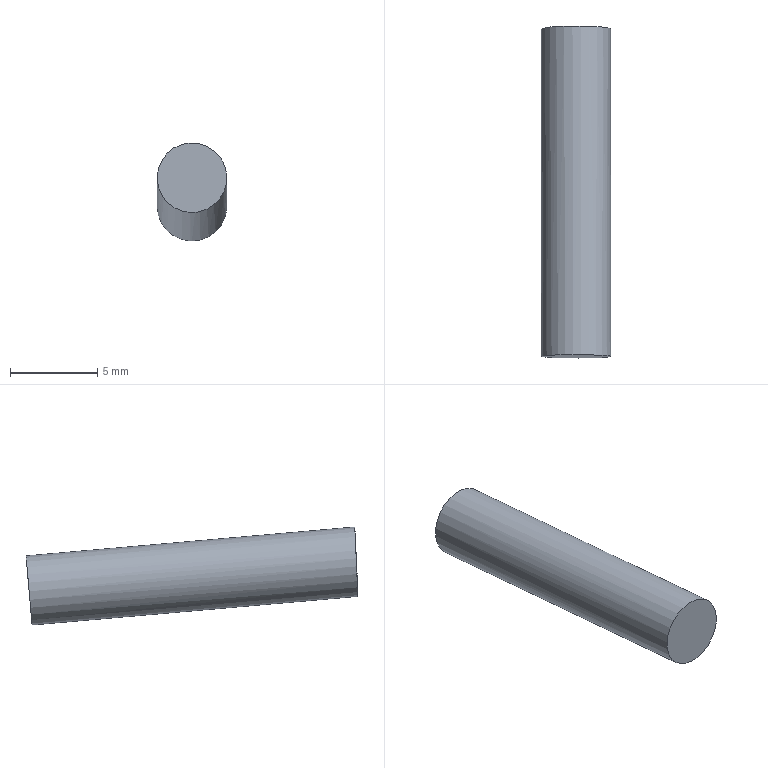Part | NX | features solid 2 | 1 solid | 3 faces | box 4 x 19.077 x 5.638 mm | volume 237.299 mm3 | plane 2 | cylinder 1 | commonest cylinder face diameters 4 x1
STEP:
#1=CARTESIAN_POINT('',(156.524,-27.849,-45.013));
#2=VERTEX_POINT('',#1);
#3=CARTESIAN_POINT('',(156.524,-27.675,-43.02));
#4=DIRECTION('',(0.,-0.9962,0.08716));
#5=DIRECTION('',(0.,-0.08716,-0.9962));
#6=AXIS2_PLACEMENT_3D('',#3,#4,#5);
#7=CIRCLE('',#6,2.);
#8=EDGE_CURVE('',#2,#2,#7,.T.);
#9=ORIENTED_EDGE('',*,*,#8,.F.);
#10=EDGE_LOOP('',(#9));
#11=FACE_BOUND('',#10,.T.);
#12=CARTESIAN_POINT('',(156.524,-27.675,-43.02));
#13=DIRECTION('',(0.,0.9962,-0.08716));
#14=DIRECTION('',(0.,0.08716,0.9962));
#15=AXIS2_PLACEMENT_3D('',#12,#13,#14);
#16=PLANE('',#15);
#17=ADVANCED_FACE('',(#11),#16,.T.);
#18=CARTESIAN_POINT('',(156.43,-46.577,-43.372));
#19=VERTEX_POINT('',#18);
#20=CARTESIAN_POINT('',(156.524,-46.487,-41.374));
#21=DIRECTION('',(0.001957,0.999,-0.04546));
#22=DIRECTION('',(-0.04675,-0.04532,-0.9979));
#23=AXIS2_PLACEMENT_3D('',#20,#21,#22);
#24=ELLIPSE('',#23,2.002,2.);
#25=EDGE_CURVE('',#19,#19,#24,.T.);
#26=ORIENTED_EDGE('',*,*,#25,.F.);
#27=EDGE_LOOP('',(#26));
#28=FACE_BOUND('',#27,.T.);
#29=CARTESIAN_POINT('',(128.811,-48.589,-88.763));
#30=DIRECTION('',(0.001957,0.999,-0.04546));
#31=DIRECTION('',(0.06617,0.04523,0.9968));
#32=AXIS2_PLACEMENT_3D('',#29,#30,#31);
#33=PLANE('',#32);
#34=ADVANCED_FACE('',(#28),#33,.F.);
#35=ORIENTED_EDGE('',*,*,#8,.T.);
#36=EDGE_LOOP('',(#35));
#37=FACE_BOUND('',#36,.T.);
#38=ORIENTED_EDGE('',*,*,#25,.T.);
#39=EDGE_LOOP('',(#38));
#40=FACE_BOUND('',#39,.T.);
#41=CARTESIAN_POINT('',(156.524,-47.599,-41.277));
#42=DIRECTION('',(0.,0.9962,-0.08716));
#43=DIRECTION('',(0.,0.08716,0.9962));
#44=AXIS2_PLACEMENT_3D('',#41,#42,#43);
#45=CYLINDRICAL_SURFACE('',#44,2.);
#46=ADVANCED_FACE('',(#37,#40),#45,.T.);
#47=CLOSED_SHELL('',(#17,#34,#46));
#48=MANIFOLD_SOLID_BREP('',#47);
#49=(LENGTH_UNIT()NAMED_UNIT(*)SI_UNIT(.MILLI.,.METRE.));
#50=UNCERTAINTY_MEASURE_WITH_UNIT(LENGTH_MEASURE(0.00001),#49,'','');
#51=(NAMED_UNIT(*)PLANE_ANGLE_UNIT()SI_UNIT($,.RADIAN.));
#52=(NAMED_UNIT(*)SI_UNIT($,.STERADIAN.)SOLID_ANGLE_UNIT());
#53=(GEOMETRIC_REPRESENTATION_CONTEXT(3)GLOBAL_UNCERTAINTY_ASSIGNED_CONTEXT((#50))GLOBAL_UNIT_ASSIGNED_CONTEXT((#49,#51,#52))REPRESENTATION_CONTEXT('',''));
#54=ADVANCED_BREP_SHAPE_REPRESENTATION('',(#48),#53);